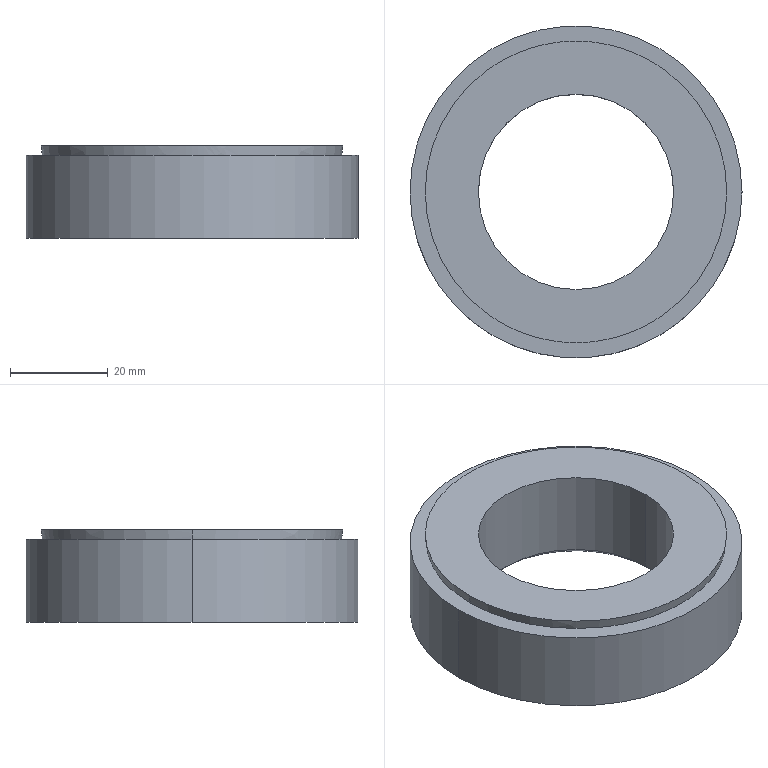Part | SolidWorks | features Chamfer 1, Extrusion 1, ICE 1, RevCut 1 | 1 solid | 11 faces | box 68 x 68 x 19 mm | volume 43740 mm3 | cylinder 4 | plane 3 | cone 2 | sphere 2 | commonest cylinder face diameters 40 x2 68 x2
STEP:
#1=CARTESIAN_POINT('',(20.,0.,1.));
#2=VERTEX_POINT('',#1);
#3=CARTESIAN_POINT('',(-20.,0.,1.));
#4=VERTEX_POINT('',#3);
#5=CARTESIAN_POINT('',(0.,0.,1.));
#6=DIRECTION('',(0.,0.,-1.));
#7=DIRECTION('',(1.,0.,0.));
#8=AXIS2_PLACEMENT_3D('',#5,#6,#7);
#9=CIRCLE('',#8,20.);
#10=EDGE_CURVE('',#2,#4,#9,.T.);
#11=ORIENTED_EDGE('',*,*,#10,.F.);
#12=CARTESIAN_POINT('',(21.,0.,0.));
#13=VERTEX_POINT('',#12);
#14=CARTESIAN_POINT('',(21.,0.,0.));
#15=DIRECTION('',(0.7071,0.,-0.7071));
#16=VECTOR('',#15,1000.);
#17=LINE('',#14,#16);
#18=EDGE_CURVE('',#2,#13,#17,.T.);
#19=ORIENTED_EDGE('',*,*,#18,.T.);
#20=CARTESIAN_POINT('',(-21.,0.,0.));
#21=VERTEX_POINT('',#20);
#22=CARTESIAN_POINT('',(0.,0.,0.));
#23=DIRECTION('',(0.,0.,1.));
#24=DIRECTION('',(1.,0.,0.));
#25=AXIS2_PLACEMENT_3D('',#22,#23,#24);
#26=CIRCLE('',#25,21.);
#27=EDGE_CURVE('',#21,#13,#26,.T.);
#28=ORIENTED_EDGE('',*,*,#27,.F.);
#29=CARTESIAN_POINT('',(-21.,0.,0.));
#30=DIRECTION('',(-0.7071,0.,-0.7071));
#31=VECTOR('',#30,1000.);
#32=LINE('',#29,#31);
#33=EDGE_CURVE('',#4,#21,#32,.T.);
#34=ORIENTED_EDGE('',*,*,#33,.F.);
#35=EDGE_LOOP('',(#11,#19,#28,#34));
#36=FACE_OUTER_BOUND('',#35,.T.);
#37=CARTESIAN_POINT('',(0.,0.,0.));
#38=DIRECTION('',(0.,0.,-1.));
#39=DIRECTION('',(-1.,0.,0.));
#40=AXIS2_PLACEMENT_3D('',#37,#38,#39);
#41=CONICAL_SURFACE('',#40,21.,0.7854);
#42=ADVANCED_FACE('',(#36),#41,.F.);
#43=ORIENTED_EDGE('',*,*,#10,.T.);
#44=CARTESIAN_POINT('',(-20.,0.,19.));
#45=VERTEX_POINT('',#44);
#46=CARTESIAN_POINT('',(-20.,0.,0.));
#47=DIRECTION('',(0.,0.,1.));
#48=VECTOR('',#47,1000.);
#49=LINE('',#46,#48);
#50=EDGE_CURVE('',#4,#45,#49,.T.);
#51=ORIENTED_EDGE('',*,*,#50,.T.);
#52=CARTESIAN_POINT('',(20.,0.,19.));
#53=VERTEX_POINT('',#52);
#54=CARTESIAN_POINT('',(0.,0.,19.));
#55=DIRECTION('',(0.,0.,1.));
#56=DIRECTION('',(1.,0.,0.));
#57=AXIS2_PLACEMENT_3D('',#54,#55,#56);
#58=CIRCLE('',#57,20.);
#59=EDGE_CURVE('',#45,#53,#58,.T.);
#60=ORIENTED_EDGE('',*,*,#59,.T.);
#61=CARTESIAN_POINT('',(20.,0.,0.));
#62=DIRECTION('',(0.,0.,1.));
#63=VECTOR('',#62,1000.);
#64=LINE('',#61,#63);
#65=EDGE_CURVE('',#2,#53,#64,.T.);
#66=ORIENTED_EDGE('',*,*,#65,.F.);
#67=EDGE_LOOP('',(#43,#51,#60,#66));
#68=FACE_OUTER_BOUND('',#67,.T.);
#69=CARTESIAN_POINT('',(0.,0.,0.));
#70=DIRECTION('',(0.,0.,1.));
#71=DIRECTION('',(1.,0.,0.));
#72=AXIS2_PLACEMENT_3D('',#69,#70,#71);
#73=CYLINDRICAL_SURFACE('',#72,20.);
#74=ADVANCED_FACE('',(#68),#73,.F.);
#75=CARTESIAN_POINT('',(-30.626,0.,17.));
#76=VERTEX_POINT('',#75);
#77=CARTESIAN_POINT('',(30.626,0.,17.));
#78=VERTEX_POINT('',#77);
#79=CARTESIAN_POINT('',(0.,0.,17.));
#80=DIRECTION('',(0.,0.,1.));
#81=DIRECTION('',(1.,0.,0.));
#82=AXIS2_PLACEMENT_3D('',#79,#80,#81);
#83=CIRCLE('',#82,30.626);
#84=EDGE_CURVE('',#76,#78,#83,.T.);
#85=ORIENTED_EDGE('',*,*,#84,.T.);
#86=CARTESIAN_POINT('',(30.873,0.,19.));
#87=VERTEX_POINT('',#86);
#88=CARTESIAN_POINT('',(0.,0.,21.8));
#89=DIRECTION('',(0.,-1.,0.));
#90=DIRECTION('',(1.,0.,0.));
#91=AXIS2_PLACEMENT_3D('',#88,#89,#90);
#92=CIRCLE('',#91,31.);
#93=EDGE_CURVE('',#78,#87,#92,.T.);
#94=ORIENTED_EDGE('',*,*,#93,.T.);
#95=CARTESIAN_POINT('',(-30.873,0.,19.));
#96=VERTEX_POINT('',#95);
#97=CARTESIAN_POINT('',(0.,0.,19.));
#98=DIRECTION('',(0.,0.,1.));
#99=DIRECTION('',(1.,0.,0.));
#100=AXIS2_PLACEMENT_3D('',#97,#98,#99);
#101=CIRCLE('',#100,30.873);
#102=EDGE_CURVE('',#96,#87,#101,.T.);
#103=ORIENTED_EDGE('',*,*,#102,.F.);
#104=CARTESIAN_POINT('',(0.,0.,21.8));
#105=DIRECTION('',(0.,1.,0.));
#106=DIRECTION('',(0.,0.,1.));
#107=AXIS2_PLACEMENT_3D('',#104,#105,#106);
#108=CIRCLE('',#107,31.);
#109=EDGE_CURVE('',#76,#96,#108,.T.);
#110=ORIENTED_EDGE('',*,*,#109,.F.);
#111=EDGE_LOOP('',(#85,#94,#103,#110));
#112=FACE_OUTER_BOUND('',#111,.T.);
#113=CARTESIAN_POINT('',(0.,0.,21.8));
#114=DIRECTION('',(0.,-1.,0.));
#115=DIRECTION('',(-1.,0.,0.));
#116=AXIS2_PLACEMENT_3D('',#113,#114,#115);
#117=SPHERICAL_SURFACE('',#116,31.);
#118=ADVANCED_FACE('',(#112),#117,.T.);
#119=CARTESIAN_POINT('',(34.,0.,17.));
#120=VERTEX_POINT('',#119);
#121=CARTESIAN_POINT('',(-34.,0.,17.));
#122=VERTEX_POINT('',#121);
#123=CARTESIAN_POINT('',(0.,0.,17.));
#124=DIRECTION('',(0.,0.,1.));
#125=DIRECTION('',(1.,0.,0.));
#126=AXIS2_PLACEMENT_3D('',#123,#124,#125);
#127=CIRCLE('',#126,34.);
#128=EDGE_CURVE('',#120,#122,#127,.T.);
#129=ORIENTED_EDGE('',*,*,#128,.F.);
#130=CARTESIAN_POINT('',(34.,0.,0.));
#131=VERTEX_POINT('',#130);
#132=CARTESIAN_POINT('',(34.,0.,19.));
#133=DIRECTION('',(0.,0.,-1.));
#134=VECTOR('',#133,1000.);
#135=LINE('',#132,#134);
#136=EDGE_CURVE('',#120,#131,#135,.T.);
#137=ORIENTED_EDGE('',*,*,#136,.T.);
#138=CARTESIAN_POINT('',(-34.,0.,0.));
#139=VERTEX_POINT('',#138);
#140=CARTESIAN_POINT('',(0.,0.,0.));
#141=DIRECTION('',(0.,0.,1.));
#142=DIRECTION('',(1.,0.,0.));
#143=AXIS2_PLACEMENT_3D('',#140,#141,#142);
#144=CIRCLE('',#143,34.);
#145=EDGE_CURVE('',#131,#139,#144,.T.);
#146=ORIENTED_EDGE('',*,*,#145,.T.);
#147=CARTESIAN_POINT('',(-34.,0.,19.));
#148=DIRECTION('',(0.,0.,-1.));
#149=VECTOR('',#148,1000.);
#150=LINE('',#147,#149);
#151=EDGE_CURVE('',#122,#139,#150,.T.);
#152=ORIENTED_EDGE('',*,*,#151,.F.);
#153=EDGE_LOOP('',(#129,#137,#146,#152));
#154=FACE_OUTER_BOUND('',#153,.T.);
#155=CARTESIAN_POINT('',(0.,0.,19.));
#156=DIRECTION('',(0.,0.,-1.));
#157=DIRECTION('',(-1.,0.,0.));
#158=AXIS2_PLACEMENT_3D('',#155,#156,#157);
#159=CYLINDRICAL_SURFACE('',#158,34.);
#160=ADVANCED_FACE('',(#154),#159,.T.);
#161=ORIENTED_EDGE('',*,*,#136,.F.);
#162=CARTESIAN_POINT('',(0.,0.,17.));
#163=DIRECTION('',(0.,0.,1.));
#164=DIRECTION('',(1.,0.,0.));
#165=AXIS2_PLACEMENT_3D('',#162,#163,#164);
#166=CIRCLE('',#165,34.);
#167=EDGE_CURVE('',#122,#120,#166,.T.);
#168=ORIENTED_EDGE('',*,*,#167,.F.);
#169=ORIENTED_EDGE('',*,*,#151,.T.);
#170=CARTESIAN_POINT('',(0.,0.,0.));
#171=DIRECTION('',(0.,0.,1.));
#172=DIRECTION('',(1.,0.,0.));
#173=AXIS2_PLACEMENT_3D('',#170,#171,#172);
#174=CIRCLE('',#173,34.);
#175=EDGE_CURVE('',#139,#131,#174,.T.);
#176=ORIENTED_EDGE('',*,*,#175,.T.);
#177=EDGE_LOOP('',(#161,#168,#169,#176));
#178=FACE_OUTER_BOUND('',#177,.T.);
#179=CARTESIAN_POINT('',(0.,0.,19.));
#180=DIRECTION('',(0.,0.,-1.));
#181=DIRECTION('',(-1.,0.,0.));
#182=AXIS2_PLACEMENT_3D('',#179,#180,#181);
#183=CYLINDRICAL_SURFACE('',#182,34.);
#184=ADVANCED_FACE('',(#178),#183,.T.);
#185=ORIENTED_EDGE('',*,*,#27,.T.);
#186=CARTESIAN_POINT('',(0.,0.,0.));
#187=DIRECTION('',(0.,0.,1.));
#188=DIRECTION('',(1.,0.,0.));
#189=AXIS2_PLACEMENT_3D('',#186,#187,#188);
#190=CIRCLE('',#189,21.);
#191=EDGE_CURVE('',#13,#21,#190,.T.);
#192=ORIENTED_EDGE('',*,*,#191,.T.);
#193=EDGE_LOOP('',(#185,#192));
#194=FACE_BOUND('',#193,.T.);
#195=ORIENTED_EDGE('',*,*,#175,.F.);
#196=ORIENTED_EDGE('',*,*,#145,.F.);
#197=EDGE_LOOP('',(#195,#196));
#198=FACE_OUTER_BOUND('',#197,.T.);
#199=CARTESIAN_POINT('',(0.,0.,0.));
#200=DIRECTION('',(0.,0.,1.));
#201=DIRECTION('',(1.,0.,0.));
#202=AXIS2_PLACEMENT_3D('',#199,#200,#201);
#203=PLANE('',#202);
#204=ADVANCED_FACE('',(#194,#198),#203,.F.);
#205=ORIENTED_EDGE('',*,*,#93,.F.);
#206=CARTESIAN_POINT('',(0.,0.,17.));
#207=DIRECTION('',(0.,0.,1.));
#208=DIRECTION('',(1.,0.,0.));
#209=AXIS2_PLACEMENT_3D('',#206,#207,#208);
#210=CIRCLE('',#209,30.626);
#211=EDGE_CURVE('',#78,#76,#210,.T.);
#212=ORIENTED_EDGE('',*,*,#211,.T.);
#213=ORIENTED_EDGE('',*,*,#109,.T.);
#214=CARTESIAN_POINT('',(0.,0.,19.));
#215=DIRECTION('',(0.,0.,1.));
#216=DIRECTION('',(1.,0.,0.));
#217=AXIS2_PLACEMENT_3D('',#214,#215,#216);
#218=CIRCLE('',#217,30.873);
#219=EDGE_CURVE('',#87,#96,#218,.T.);
#220=ORIENTED_EDGE('',*,*,#219,.F.);
#221=EDGE_LOOP('',(#205,#212,#213,#220));
#222=FACE_OUTER_BOUND('',#221,.T.);
#223=CARTESIAN_POINT('',(0.,0.,21.8));
#224=DIRECTION('',(0.,-1.,0.));
#225=DIRECTION('',(-1.,0.,0.));
#226=AXIS2_PLACEMENT_3D('',#223,#224,#225);
#227=SPHERICAL_SURFACE('',#226,31.);
#228=ADVANCED_FACE('',(#222),#227,.T.);
#229=ORIENTED_EDGE('',*,*,#167,.T.);
#230=ORIENTED_EDGE('',*,*,#128,.T.);
#231=EDGE_LOOP('',(#229,#230));
#232=FACE_OUTER_BOUND('',#231,.T.);
#233=ORIENTED_EDGE('',*,*,#84,.F.);
#234=ORIENTED_EDGE('',*,*,#211,.F.);
#235=EDGE_LOOP('',(#233,#234));
#236=FACE_BOUND('',#235,.T.);
#237=CARTESIAN_POINT('',(-34.,0.,17.));
#238=DIRECTION('',(0.,0.,1.));
#239=DIRECTION('',(1.,0.,0.));
#240=AXIS2_PLACEMENT_3D('',#237,#238,#239);
#241=PLANE('',#240);
#242=ADVANCED_FACE('',(#232,#236),#241,.T.);
#243=CARTESIAN_POINT('',(0.,0.,19.));
#244=DIRECTION('',(0.,0.,1.));
#245=DIRECTION('',(1.,0.,0.));
#246=AXIS2_PLACEMENT_3D('',#243,#244,#245);
#247=CIRCLE('',#246,20.);
#248=EDGE_CURVE('',#53,#45,#247,.T.);
#249=ORIENTED_EDGE('',*,*,#248,.F.);
#250=ORIENTED_EDGE('',*,*,#59,.F.);
#251=EDGE_LOOP('',(#249,#250));
#252=FACE_BOUND('',#251,.T.);
#253=ORIENTED_EDGE('',*,*,#102,.T.);
#254=ORIENTED_EDGE('',*,*,#219,.T.);
#255=EDGE_LOOP('',(#253,#254));
#256=FACE_OUTER_BOUND('',#255,.T.);
#257=CARTESIAN_POINT('',(0.,0.,19.));
#258=DIRECTION('',(0.,0.,1.));
#259=DIRECTION('',(1.,0.,0.));
#260=AXIS2_PLACEMENT_3D('',#257,#258,#259);
#261=PLANE('',#260);
#262=ADVANCED_FACE('',(#252,#256),#261,.T.);
#263=ORIENTED_EDGE('',*,*,#50,.F.);
#264=CARTESIAN_POINT('',(0.,0.,1.));
#265=DIRECTION('',(0.,0.,-1.));
#266=DIRECTION('',(1.,0.,0.));
#267=AXIS2_PLACEMENT_3D('',#264,#265,#266);
#268=CIRCLE('',#267,20.);
#269=EDGE_CURVE('',#4,#2,#268,.T.);
#270=ORIENTED_EDGE('',*,*,#269,.T.);
#271=ORIENTED_EDGE('',*,*,#65,.T.);
#272=ORIENTED_EDGE('',*,*,#248,.T.);
#273=EDGE_LOOP('',(#263,#270,#271,#272));
#274=FACE_OUTER_BOUND('',#273,.T.);
#275=CARTESIAN_POINT('',(0.,0.,0.));
#276=DIRECTION('',(0.,0.,1.));
#277=DIRECTION('',(1.,0.,0.));
#278=AXIS2_PLACEMENT_3D('',#275,#276,#277);
#279=CYLINDRICAL_SURFACE('',#278,20.);
#280=ADVANCED_FACE('',(#274),#279,.F.);
#281=ORIENTED_EDGE('',*,*,#18,.F.);
#282=ORIENTED_EDGE('',*,*,#269,.F.);
#283=ORIENTED_EDGE('',*,*,#33,.T.);
#284=ORIENTED_EDGE('',*,*,#191,.F.);
#285=EDGE_LOOP('',(#281,#282,#283,#284));
#286=FACE_OUTER_BOUND('',#285,.T.);
#287=CARTESIAN_POINT('',(0.,0.,0.));
#288=DIRECTION('',(0.,0.,-1.));
#289=DIRECTION('',(-1.,0.,0.));
#290=AXIS2_PLACEMENT_3D('',#287,#288,#289);
#291=CONICAL_SURFACE('',#290,21.,0.7854);
#292=ADVANCED_FACE('',(#286),#291,.F.);
#293=CLOSED_SHELL('',(#42,#74,#118,#160,#184,#204,#228,#242,#262,#280,#292));
#294=MANIFOLD_SOLID_BREP('',#293);
#295=CARTESIAN_POINT('',(0.,0.,0.));
#296=DIRECTION('',(0.,0.,1.));
#297=DIRECTION('',(1.,0.,0.));
#298=AXIS2_PLACEMENT_3D('',#295,#296,#297);
#299=(LENGTH_UNIT()NAMED_UNIT(*)SI_UNIT(.MILLI.,.METRE.));
#300=UNCERTAINTY_MEASURE_WITH_UNIT(LENGTH_MEASURE(0.00001),#299,'','');
#301=(NAMED_UNIT(*)PLANE_ANGLE_UNIT()SI_UNIT($,.RADIAN.));
#302=(NAMED_UNIT(*)SI_UNIT($,.STERADIAN.)SOLID_ANGLE_UNIT());
#303=(GEOMETRIC_REPRESENTATION_CONTEXT(3)GLOBAL_UNCERTAINTY_ASSIGNED_CONTEXT((#300))GLOBAL_UNIT_ASSIGNED_CONTEXT((#299,#301,#302))REPRESENTATION_CONTEXT('',''));
#304=ADVANCED_BREP_SHAPE_REPRESENTATION('',(#294,#298),#303);